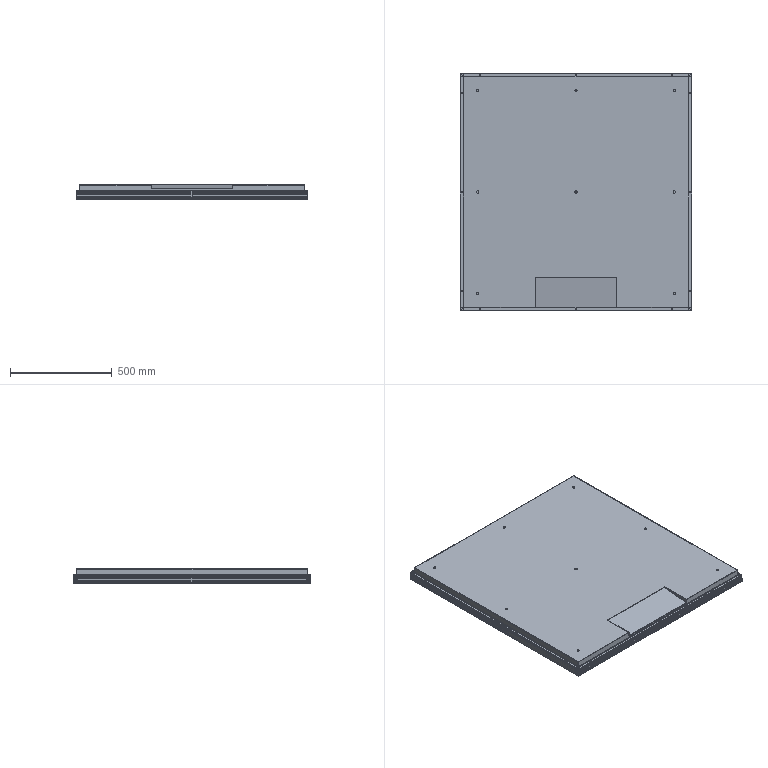Part | 9 solids | 560 faces | box 1140 x 1170 x 70.147 mm | volume 17306974 mm3 | plane 344 | cylinder 204 | spline 12 | commonest cylinder face diameters 0.6 x80 4 x34 7 x30 3 x16 11 x16 0.4 x9